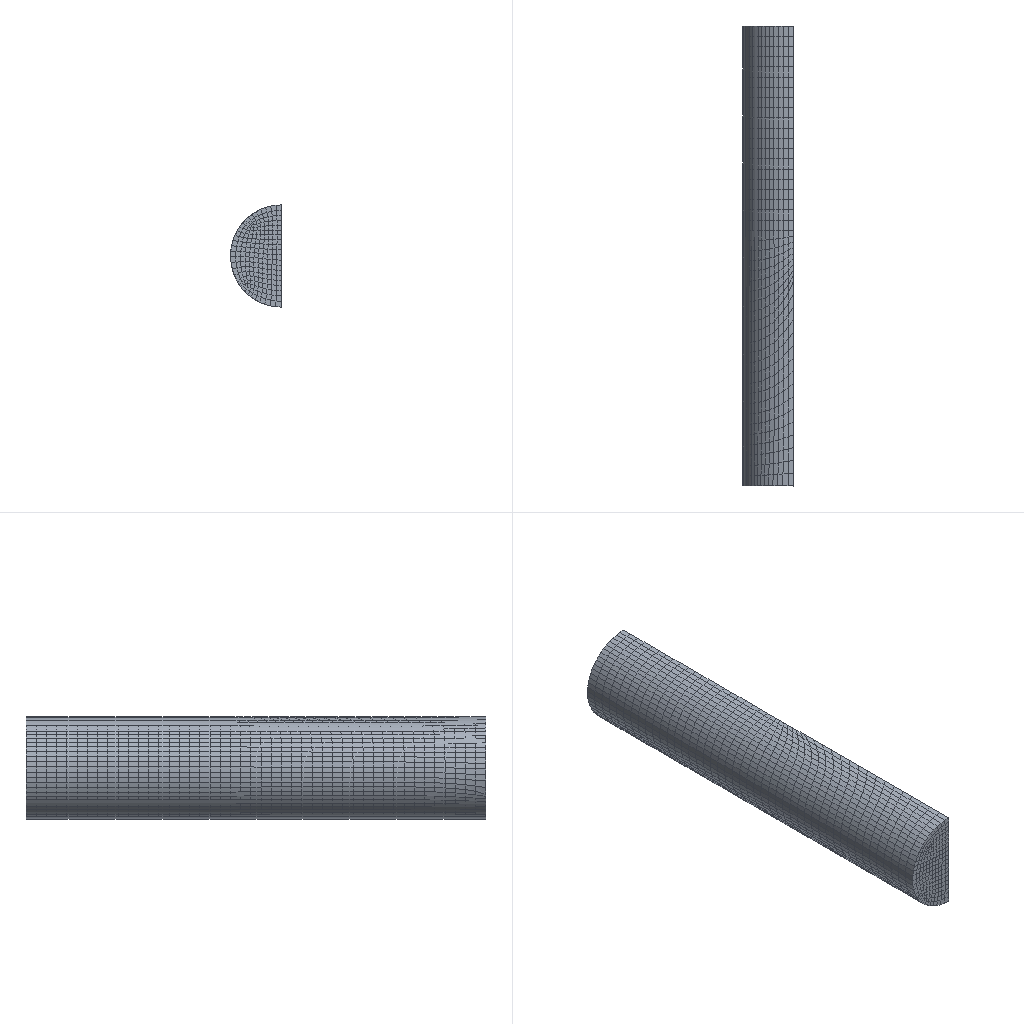Simulation study | abaqus
Set-up summary:
category,name,step,type,value,unit,region
solver,abaqus
solver,version,,,Abaqus/Explicit 2020
units,not stated in the deck,,not stated
analysis,deck,,transient,transient
load_step,Step-1,Step-1,transient
load_step,requested,,,1
mesh,nodes,,,21434
mesh,elements,,,32778
element_type,C3D4,,solid,18187
element_type,R3D3,,rigid,116
element_type,R3D4,,rigid,5160
element_type,EC3D8R,,solid,9315
load,load commands in deck,,count,2
bc,support commands in deck,,count,11
material,MATERIAL-1,,in results
material,SIC,,in results
check,setup vs results,,match,"per instance, exact: element labels, types and connectivity; labels of the nodes the elements use; coordinates of those nodes at SINGLE_PRECISION in 3 of 4 instance(s)"
Abaqus input file, long lists of numbers shortened:
*Heading
** Job name: Job-1 Model name: Model-1
** Generated by: Abaqus/CAE 2020
*Preprint, echo=NO, model=NO, history=NO, contact=NO
**
** PARTS
**
*Part, name=Parricles
*Node
      1,   11.255,   1.909,   46.552
      2,   12.345,   4.467,   50.813
** (5446 more lines like these left out)
*Element, type=C3D4
  1, 3764, 3765, 3766, 3767
  2, 3767, 3764, 3768, 3769
** (18185 more lines like these left out)
*Nset, nset=Set-1, generate
    1,  5448,     1
*Elset, elset=Set-1, generate
     1,  18187,      1
** Section: keli
*Solid Section, elset=Set-1, material=sic
,
*End Part
**
*Part, name=jiya-2
*Node
      1,  -15.69,   -19.323,  -107.129
      2,  -15.69,   120.677,  -107.129
** (4349 more lines like these left out)
*Element, type=R3D4
  1,    1,   87,  768,  775
  2,   87,   88,  769,  768
** (4296 more lines like these left out)
*Element, type=R3D3
2959, 3225,  104,  103
2960, 3221,  101,    3
** (104 more lines like these left out)
*Node
   4352, 5.81707246e-15,   120.677,         -75.
*Nset, nset=jiya-2-RefPt_, internal
4352,
*Elset, elset=jiya-2, generate
    1,  4404,     1
*End Part
**
*Part, name=jiya-18
*Node
      1,          20.,   165.677,         -75.
      2,          20.,   80.677,         -75.
** (867 more lines like these left out)
*Element, type=R3D4
  1,   1,  32,  63,  93
  2,  32,  31,  64,  63
** (860 more lines like these left out)
*Element, type=R3D3
652, 738, 749, 747
653, 760, 704, 767
** (8 more lines like these left out)
*Node
    870,           0.,   165.677,         -75.
*Nset, nset=jiya-18-RefPt_, internal
870,
*Elset, elset=jiya-18, generate
   1,  872,    1
*End Part
**
*Part, name=oula
*Node
      1,    20.,  -0.1182,         -20.
      2,   -20.,  -0.1182,         -20.
** (10762 more lines like these left out)
*Element, type=EC3D8R
   1,   11,   12,  272,  270, 1352, 1353, 2968, 2966
   2,   12,   13,  273,  272, 1353, 1354, 2969, 2968
** (9313 more lines like these left out)
*Nset, nset=Set-3, generate
     1,  10764,      1
*Elset, elset=Set-3, generate
    1,  9315,     1
** Section: Section-1
*Eulerian Section, elset=Set-3
Material-1, material-1-1
*Surface, type=EULERIAN MATERIAL, name=material-1-1
material-1-1
*End Part
**
**
** ASSEMBLY
**
*Assembly, name=Assembly
**
*Instance, name=jiya-2-1, part=jiya-2
*End Instance
**
*Instance, name=jiya-18-1, part=jiya-18
*End Instance
**
*Instance, name=oula-1, part=oula
    0.1182,   -19.323,         -75.
    0.1182,   -19.323,         -75., 0.6955, -18.746, -75.577,         120.
*End Instance
**
*Instance, name=Parricles-1, part=Parricles
        -15.,          80.,         -61.
        -15.,          80.,         -61., -14.423, 80.577, -61.577,         120.
*End Instance
**
*Nset, nset=Set-1, instance=jiya-2-1
    4,    6,   17,   18,   21,   22,   25,   26,   36,   40,   41,   44,  108,  109,  110,  111
  112,  113,  114,  122,  123,  124,  125,  126,  127,  128,  189,  190,  191,  197,  198,  199
** (23 more lines like these left out)
*Elset, elset=Set-1, instance=jiya-2-1, generate
 3989,  4354,     1
*Nset, nset=Set-2, instance=oula-1, generate
     1,  10764,      1
*Nset, nset=Set-2, instance=Parricles-1, generate
    1,  5448,     1
*Elset, elset=Set-2, instance=oula-1, generate
    1,  9315,     1
*Elset, elset=Set-2, instance=Parricles-1, generate
     1,  18187,      1
*Nset, nset=Set-3, instance=jiya-2-1
 4352,
*Nset, nset=Set-4, instance=oula-1
    1,    2,    3,    4,    6,    7,    8,    9,   10,   11,   12,   13,   14,   15,   16,   17
   18,   19,   20,   21,   22,   23,   24,   25,   26,   27,   28,   60,   61,   62,   63,   64
** (59 more lines like these left out)
*Elset, elset=Set-4, instance=oula-1
    1,    2,    3,    4,    5,    6,    7,    8,    9,   10,  119,  128,  151,  159,  167,  175
  183,  184,  185,  186,  208,  209,  210,  211,  212,  213,  214,  215,  216,  217,  326,  335
** (55 more lines like these left out)
*Nset, nset=Set-5, instance=oula-1
    1,    2,    3,    4,    5,    6,    7,   29,   30,   31,   32,   33,   34,   35,   36,   37
   38,   39,   40,   41,   42,   43,   44,   45,   46,   47,   48,   49,   50,   51,   52,   53
** (52 more lines like these left out)
*Elset, elset=Set-5, instance=oula-1
   92,   94,   96,   98,  100,  102,  104,  106,  108,  110,  111,  112,  113,  114,  115,  116
  117,  118,  119,  129,  130,  131,  132,  133,  186,  189,  192,  195,  198,  201,  204,  207
** (48 more lines like these left out)
*Nset, nset=Set-6, instance=oula-1
   3,   4,   5, 106, 107, 108, 109, 110, 111, 112, 113, 114, 115, 116, 117, 118
 119, 120, 121, 122, 123, 124, 125, 126, 127, 128, 129, 130, 131, 132, 133, 134
** (13 more lines like these left out)
*Elset, elset=Set-6, instance=oula-1, generate
 4969,  5175,     1
*Nset, nset=Set-7, instance=oula-1
     1,     2,     8,     9,    10,    11,    12,    13,    14,    15,    16,    17,    18,    19,    20,    21
    22,    23,    24,    25,    26,    27,    28,    29,    30,    31,    32,    33,    34,    35,    36,    37
** (306 more lines like these left out)
*Elset, elset=Set-7, instance=oula-1, generate
 5176,  9315,     1
*Nset, nset=Set-9, instance=oula-1
   3,   4,   5, 106, 107, 108, 109, 110, 111, 112, 113, 114, 115, 116, 117, 118
 119, 120, 121, 122, 123, 124, 125, 126, 127, 128, 129, 130, 131, 132, 133, 134
** (13 more lines like these left out)
*Elset, elset=Set-9, instance=oula-1, generate
 4969,  5175,     1
*Nset, nset=Set-10, instance=oula-1
    1,    2,    3,    4,    6,    7,    8,    9,   10,   11,   12,   13,   14,   15,   16,   17
   18,   19,   20,   21,   22,   23,   24,   25,   26,   27,   28,   60,   61,   62,   63,   64
** (59 more lines like these left out)
*Elset, elset=Set-10, instance=oula-1
    1,    2,    3,    4,    5,    6,    7,    8,    9,   10,  119,  128,  151,  159,  167,  175
  183,  184,  185,  186,  208,  209,  210,  211,  212,  213,  214,  215,  216,  217,  326,  335
** (55 more lines like these left out)
*Nset, nset=Set-11, instance=oula-1
    1,    2,    3,    4,    5,    6,    7,    8,    9,   29,   30,   31,   32,   33,   34,   35
   36,   37,   38,   39,   40,   41,   42,   43,   44,   45,   46,   47,   48,   49,   50,   51
** (93 more lines like these left out)
*Elset, elset=Set-11, instance=oula-1
   92,   94,   96,   98,  100,  102,  104,  106,  108,  110,  111,  112,  113,  114,  115,  116
  117,  118,  119,  129,  130,  131,  132,  133,  186,  189,  192,  195,  198,  201,  204,  207
** (88 more lines like these left out)
*Nset, nset=Set-13, instance=jiya-18-1
 870,
*Nset, nset=m_Set-14, instance=Parricles-1, generate
    1,  5448,     1
*Elset, elset=m_Set-14, instance=Parricles-1, generate
     1,  18187,      1
*Nset, nset=s_Set-14, instance=oula-1
     1,     2,     8,     9,    10,    11,    12,    13,    14,    15,    16,    17,    18,    19,    20,    21
    22,    23,    24,    25,    26,    27,    28,    29,    30,    31,    32,    33,    34,    35,    36,    37
** (306 more lines like these left out)
*Elset, elset=s_Set-14, instance=oula-1, generate
 5176,  9315,     1
*Nset, nset=s_Set-16, instance=oula-1, generate
     1,  10764,      1
*Elset, elset=s_Set-16, instance=oula-1, generate
    1,  9315,     1
*Rigid Body, ref node=jiya-2-1.jiya-2-RefPt_, elset=jiya-2-1.jiya-2
*Rigid Body, ref node=jiya-18-1.jiya-18-RefPt_, elset=jiya-18-1.jiya-18
*End Assembly
**
** MATERIALS
**
*Material, name=Material-1
*Density
 2e-09,
*Elastic
50000., 0.35
*Plastic
300.,  0.
350., 0.1
*Material, name=sic
*Density
 3e-09,
*Elastic
150000., 0.28
**
** INTERACTION PROPERTIES
**
*Surface Interaction, name=IntProp-1
*Friction
 0.1,
*Surface Behavior, pressure-overclosure=HARD
**
** PREDEFINED FIELDS
**
** Name: Predefined Field-2   Type: Material assignment
*Initial Conditions, type=VOLUME FRACTION
Set-7, oula-1.material-1-1, 1.
** ----------------------------------------------------------------
**
** STEP: Step-1
**
*Step, name=Step-1, nlgeom=YES
*Dynamic, Explicit
, 0.001
*Bulk Viscosity
0.06, 1.2
** Mass Scaling: Semi-Automatic
**               Whole Model
*Fixed Mass Scaling, dt=1e-07, type=below min
**
** BOUNDARY CONDITIONS
**
** Name: BC-1 Type: 对称/反对称/完全固定
*Boundary
Set-3, ENCASTRE
** Name: [REDACTED]
*Boundary, type=VELOCITY
Set-9, 2, 2
** Name: [REDACTED]
*Boundary, type=VELOCITY
Set-10, 1, 1
** Name: [REDACTED]
*Boundary, type=VELOCITY
Set-11, 1, 1
Set-11, 3, 3
** Name: [REDACTED] : Speed/Angular velocity
*Boundary, type=VELOCITY
Set-13, 1, 1
Set-13, 2, 2, -50000.
Set-13, 3, 3
Set-13, 4, 4
Set-13, 5, 5
Set-13, 6, 6
**
** PREDEFINED FIELDS
**
** Name: Predefined Field-1   Type: Temperature
*Temperature
Set-2, 350.
**
** INTERACTIONS
**
** Interaction: Int-1
*Contact, op=NEW
*Contact Inclusions, ALL EXTERIOR
*Contact Property Assignment
 ,  , IntProp-1
**
** OUTPUT REQUESTS
**
*Restart, write, number interval=1, time marks=NO
**
** FIELD OUTPUT: F-Output-1
**
*Output, field, number interval=50
*Node Output
A, AR, AT, CF, RF, RM, RT, U
UR, UT, V, VR, VT
*Element Output, directions=YES
DENSITYVAVG, E, ESDV, ESOL, EVF, EVOL, FV, LE, MISES, MISESMAX, MISESONLY, PE, PEEQ, PEEQMAX, PEEQT, PEEQVAVG
PEMAG, PEVAVG, S, SDV, SF, SSAVG, SVAVG, SVOL, TEMP, TEMPMAVG, TSHR, VEEQ, YIELDPOT
*Contact Output
CDISP, CSTRESS
**
** HISTORY OUTPUT: H-Output-1
**
*Output, history, variable=PRESELECT
*End Step
Results summary:
result,step,Step-1,partial,increments=8498 time=0.0007571/0.001
result,analysis,,,transient
result,last_loadstep,,,1
result,primary field,,,U
result,reaction total,,FX,-6605.484,model units
result,reaction total,,FY,56412.625,model units
result,reaction total,,FZ,-18955.117,model units